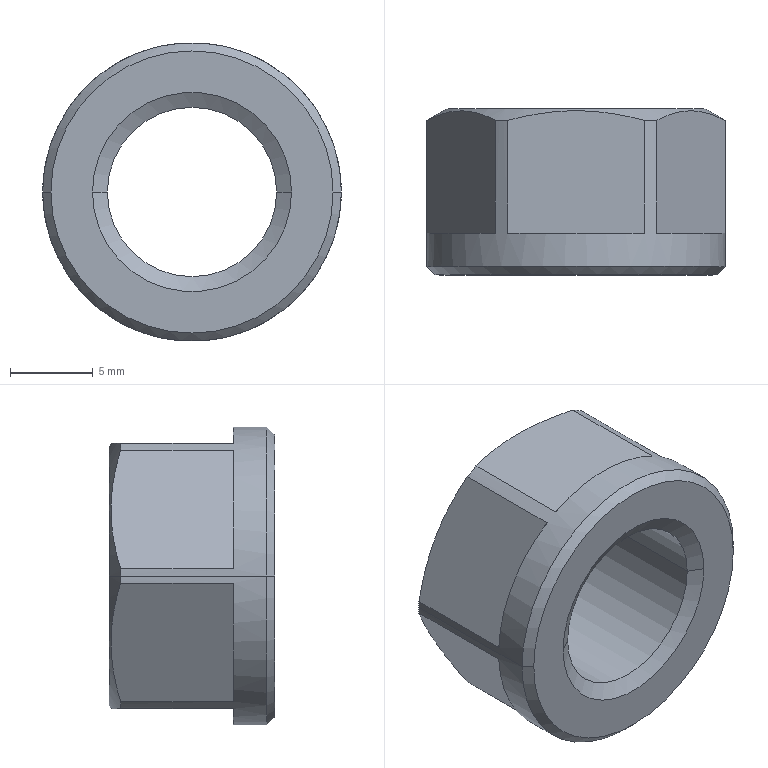Part | SolidWorks | features BaseBody 1 | 1 solid | 26 faces | box 18 x 10 x 18 mm | volume 1447 mm3 | plane 14 | cone 8 | cylinder 4 | commonest cylinder face diameters 10.2 x2 18 x2
STEP:
#1=CARTESIAN_POINT('',(59.,179.1,-24.25));
#2=VERTEX_POINT('',#1);
#3=CARTESIAN_POINT('',(42.,179.1,-24.25));
#4=VERTEX_POINT('',#3);
#5=CARTESIAN_POINT('',(50.5,179.1,-24.25));
#6=DIRECTION('',(0.,-1.,0.));
#7=DIRECTION('',(-1.,0.,0.));
#8=AXIS2_PLACEMENT_3D('',#5,#6,#7);
#9=CIRCLE('',#8,8.5);
#10=EDGE_CURVE('',#2,#4,#9,.T.);
#11=ORIENTED_EDGE('',*,*,#10,.F.);
#12=CARTESIAN_POINT('',(59.5,179.6,-24.25));
#13=VERTEX_POINT('',#12);
#14=CARTESIAN_POINT('',(59.5,179.6,-24.25));
#15=DIRECTION('',(0.7071,0.7071,0.));
#16=VECTOR('',#15,1000.);
#17=LINE('',#14,#16);
#18=EDGE_CURVE('',#2,#13,#17,.T.);
#19=ORIENTED_EDGE('',*,*,#18,.T.);
#20=CARTESIAN_POINT('',(41.5,179.6,-24.25));
#21=VERTEX_POINT('',#20);
#22=CARTESIAN_POINT('',(50.5,179.6,-24.25));
#23=DIRECTION('',(0.,1.,0.));
#24=DIRECTION('',(-1.,0.,0.));
#25=AXIS2_PLACEMENT_3D('',#22,#23,#24);
#26=CIRCLE('',#25,9.);
#27=EDGE_CURVE('',#21,#13,#26,.T.);
#28=ORIENTED_EDGE('',*,*,#27,.F.);
#29=CARTESIAN_POINT('',(41.5,179.6,-24.25));
#30=DIRECTION('',(-0.7071,0.7071,0.));
#31=VECTOR('',#30,1000.);
#32=LINE('',#29,#31);
#33=EDGE_CURVE('',#4,#21,#32,.T.);
#34=ORIENTED_EDGE('',*,*,#33,.F.);
#35=EDGE_LOOP('',(#11,#19,#28,#34));
#36=FACE_OUTER_BOUND('',#35,.T.);
#37=CARTESIAN_POINT('',(50.5,179.6,-24.25));
#38=DIRECTION('',(0.,1.,0.));
#39=DIRECTION('',(-1.,0.,0.));
#40=AXIS2_PLACEMENT_3D('',#37,#38,#39);
#41=CONICAL_SURFACE('',#40,9.,0.7854);
#42=ADVANCED_FACE('',(#36),#41,.T.);
#43=CARTESIAN_POINT('',(58.294,189.1,-24.25));
#44=VERTEX_POINT('',#43);
#45=CARTESIAN_POINT('',(42.706,189.1,-24.25));
#46=VERTEX_POINT('',#45);
#47=CARTESIAN_POINT('',(50.5,189.1,-24.25));
#48=DIRECTION('',(0.,1.,0.));
#49=DIRECTION('',(-1.,0.,0.));
#50=AXIS2_PLACEMENT_3D('',#47,#48,#49);
#51=CIRCLE('',#50,7.794);
#52=EDGE_CURVE('',#44,#46,#51,.T.);
#53=ORIENTED_EDGE('',*,*,#52,.F.);
#54=CARTESIAN_POINT('',(59.5,188.404,-24.25));
#55=VERTEX_POINT('',#54);
#56=CARTESIAN_POINT('',(58.294,189.1,-24.25));
#57=DIRECTION('',(0.866,-0.5,0.));
#58=VECTOR('',#57,1000.);
#59=LINE('',#56,#58);
#60=EDGE_CURVE('',#44,#55,#59,.T.);
#61=ORIENTED_EDGE('',*,*,#60,.T.);
#62=CARTESIAN_POINT('',(59.49,188.404,-24.679));
#63=VERTEX_POINT('',#62);
#64=CARTESIAN_POINT('',(50.5,188.404,-24.25));
#65=DIRECTION('',(0.,1.,0.));
#66=DIRECTION('',(1.,0.,0.));
#67=AXIS2_PLACEMENT_3D('',#64,#65,#66);
#68=CIRCLE('',#67,9.);
#69=EDGE_CURVE('',#55,#63,#68,.T.);
#70=ORIENTED_EDGE('',*,*,#69,.T.);
#71=CARTESIAN_POINT('',(55.367,188.404,-31.821));
#72=VERTEX_POINT('',#71);
#73=CARTESIAN_POINT('',(59.49,188.404,-24.679));
#74=CARTESIAN_POINT('',(59.152,188.582,-25.264));
#75=CARTESIAN_POINT('',(58.812,188.727,-25.852));
#76=CARTESIAN_POINT('',(58.128,188.927,-27.038));
#77=CARTESIAN_POINT('',(57.783,188.981,-27.636));
#78=CARTESIAN_POINT('',(57.261,188.982,-28.54));
#79=CARTESIAN_POINT('',(57.086,188.969,-28.843));
#80=CARTESIAN_POINT('',(56.737,188.917,-29.448));
#81=CARTESIAN_POINT('',(56.563,188.878,-29.748));
#82=CARTESIAN_POINT('',(56.046,188.728,-30.644));
#83=CARTESIAN_POINT('',(55.705,188.583,-31.235));
#84=CARTESIAN_POINT('',(55.367,188.404,-31.821));
#85=B_SPLINE_CURVE_WITH_KNOTS('',3,(#73,#74,#75,#76,#77,#78,#79,#80,#81,#82,#83,#84),.UNSPECIFIED.,.F.,.F.,(4,2,2,2,2,4),(0.000000296,0.002075,0.004149,0.005186,0.006223,0.008298),.UNSPECIFIED.);
#86=EDGE_CURVE('',#63,#72,#85,.T.);
#87=ORIENTED_EDGE('',*,*,#86,.T.);
#88=CARTESIAN_POINT('',(54.623,188.404,-32.25));
#89=VERTEX_POINT('',#88);
#90=CARTESIAN_POINT('',(50.5,188.404,-24.25));
#91=DIRECTION('',(0.,1.,0.));
#92=DIRECTION('',(1.,0.,0.));
#93=AXIS2_PLACEMENT_3D('',#90,#91,#92);
#94=CIRCLE('',#93,9.);
#95=EDGE_CURVE('',#72,#89,#94,.T.);
#96=ORIENTED_EDGE('',*,*,#95,.T.);
#97=CARTESIAN_POINT('',(46.377,188.404,-32.25));
#98=VERTEX_POINT('',#97);
#99=CARTESIAN_POINT('',(54.623,188.404,-32.25));
#100=CARTESIAN_POINT('',(53.948,188.582,-32.25));
#101=CARTESIAN_POINT('',(53.268,188.727,-32.25));
#102=CARTESIAN_POINT('',(51.899,188.927,-32.25));
#103=CARTESIAN_POINT('',(51.21,188.981,-32.25));
#104=CARTESIAN_POINT('',(50.166,188.982,-32.25));
#105=CARTESIAN_POINT('',(49.815,188.969,-32.25));
#106=CARTESIAN_POINT('',(49.117,188.917,-32.25));
#107=CARTESIAN_POINT('',(48.77,188.878,-32.25));
#108=CARTESIAN_POINT('',(47.736,188.728,-32.25));
#109=CARTESIAN_POINT('',(47.054,188.583,-32.25));
#110=CARTESIAN_POINT('',(46.377,188.404,-32.25));
#111=B_SPLINE_CURVE_WITH_KNOTS('',3,(#99,#100,#101,#102,#103,#104,#105,#106,#107,#108,#109,#110),.UNSPECIFIED.,.F.,.F.,(4,2,2,2,2,4),(0.000000256,0.002075,0.004149,0.005186,0.006223,0.008298),.UNSPECIFIED.);
#112=EDGE_CURVE('',#89,#98,#111,.T.);
#113=ORIENTED_EDGE('',*,*,#112,.T.);
#114=CARTESIAN_POINT('',(45.633,188.404,-31.821));
#115=VERTEX_POINT('',#114);
#116=CARTESIAN_POINT('',(50.5,188.404,-24.25));
#117=DIRECTION('',(0.,1.,0.));
#118=DIRECTION('',(1.,0.,0.));
#119=AXIS2_PLACEMENT_3D('',#116,#117,#118);
#120=CIRCLE('',#119,9.);
#121=EDGE_CURVE('',#98,#115,#120,.T.);
#122=ORIENTED_EDGE('',*,*,#121,.T.);
#123=CARTESIAN_POINT('',(41.51,188.404,-24.679));
#124=VERTEX_POINT('',#123);
#125=CARTESIAN_POINT('',(45.633,188.404,-31.821));
#126=CARTESIAN_POINT('',(45.296,188.582,-31.236));
#127=CARTESIAN_POINT('',(44.956,188.727,-30.648));
#128=CARTESIAN_POINT('',(44.271,188.927,-29.462));
#129=CARTESIAN_POINT('',(43.927,188.981,-28.864));
#130=CARTESIAN_POINT('',(43.405,188.982,-27.96));
#131=CARTESIAN_POINT('',(43.229,188.969,-27.657));
#132=CARTESIAN_POINT('',(42.88,188.917,-27.052));
#133=CARTESIAN_POINT('',(42.707,188.878,-26.752));
#134=CARTESIAN_POINT('',(42.19,188.728,-25.856));
#135=CARTESIAN_POINT('',(41.849,188.583,-25.265));
#136=CARTESIAN_POINT('',(41.51,188.404,-24.679));
#137=B_SPLINE_CURVE_WITH_KNOTS('',3,(#125,#126,#127,#128,#129,#130,#131,#132,#133,#134,#135,#136),.UNSPECIFIED.,.F.,.F.,(4,2,2,2,2,4),(0.000000296,0.002075,0.004149,0.005186,0.006223,0.008298),.UNSPECIFIED.);
#138=EDGE_CURVE('',#115,#124,#137,.T.);
#139=ORIENTED_EDGE('',*,*,#138,.T.);
#140=CARTESIAN_POINT('',(41.5,188.404,-24.25));
#141=VERTEX_POINT('',#140);
#142=CARTESIAN_POINT('',(50.5,188.404,-24.25));
#143=DIRECTION('',(0.,1.,0.));
#144=DIRECTION('',(1.,0.,0.));
#145=AXIS2_PLACEMENT_3D('',#142,#143,#144);
#146=CIRCLE('',#145,9.);
#147=EDGE_CURVE('',#124,#141,#146,.T.);
#148=ORIENTED_EDGE('',*,*,#147,.T.);
#149=CARTESIAN_POINT('',(42.706,189.1,-24.25));
#150=DIRECTION('',(-0.866,-0.5,0.));
#151=VECTOR('',#150,1000.);
#152=LINE('',#149,#151);
#153=EDGE_CURVE('',#46,#141,#152,.T.);
#154=ORIENTED_EDGE('',*,*,#153,.F.);
#155=EDGE_LOOP('',(#53,#61,#70,#87,#96,#113,#122,#139,#148,#154));
#156=FACE_OUTER_BOUND('',#155,.T.);
#157=CARTESIAN_POINT('',(50.5,189.1,-24.25));
#158=DIRECTION('',(0.,-1.,0.));
#159=DIRECTION('',(-1.,0.,0.));
#160=AXIS2_PLACEMENT_3D('',#157,#158,#159);
#161=CONICAL_SURFACE('',#160,7.794,1.047);
#162=ADVANCED_FACE('',(#156),#161,.T.);
#163=CARTESIAN_POINT('',(55.6,179.62,-24.25));
#164=VERTEX_POINT('',#163);
#165=CARTESIAN_POINT('',(45.4,179.62,-24.25));
#166=VERTEX_POINT('',#165);
#167=CARTESIAN_POINT('',(50.5,179.62,-24.25));
#168=DIRECTION('',(0.,1.,0.));
#169=DIRECTION('',(-1.,0.,0.));
#170=AXIS2_PLACEMENT_3D('',#167,#168,#169);
#171=CIRCLE('',#170,5.1);
#172=EDGE_CURVE('',#164,#166,#171,.T.);
#173=ORIENTED_EDGE('',*,*,#172,.T.);
#174=CARTESIAN_POINT('',(44.5,179.1,-24.25));
#175=VERTEX_POINT('',#174);
#176=CARTESIAN_POINT('',(45.4,179.62,-24.25));
#177=DIRECTION('',(-0.866,-0.5,0.));
#178=VECTOR('',#177,1000.);
#179=LINE('',#176,#178);
#180=EDGE_CURVE('',#166,#175,#179,.T.);
#181=ORIENTED_EDGE('',*,*,#180,.T.);
#182=CARTESIAN_POINT('',(56.5,179.1,-24.25));
#183=VERTEX_POINT('',#182);
#184=CARTESIAN_POINT('',(50.5,179.1,-24.25));
#185=DIRECTION('',(0.,1.,0.));
#186=DIRECTION('',(-1.,0.,0.));
#187=AXIS2_PLACEMENT_3D('',#184,#185,#186);
#188=CIRCLE('',#187,6.);
#189=EDGE_CURVE('',#183,#175,#188,.T.);
#190=ORIENTED_EDGE('',*,*,#189,.F.);
#191=CARTESIAN_POINT('',(55.6,179.62,-24.25));
#192=DIRECTION('',(0.866,-0.5,0.));
#193=VECTOR('',#192,1000.);
#194=LINE('',#191,#193);
#195=EDGE_CURVE('',#164,#183,#194,.T.);
#196=ORIENTED_EDGE('',*,*,#195,.F.);
#197=EDGE_LOOP('',(#173,#181,#190,#196));
#198=FACE_OUTER_BOUND('',#197,.T.);
#199=CARTESIAN_POINT('',(50.5,179.62,-24.25));
#200=DIRECTION('',(0.,-1.,0.));
#201=DIRECTION('',(1.,0.,0.));
#202=AXIS2_PLACEMENT_3D('',#199,#200,#201);
#203=CONICAL_SURFACE('',#202,5.1,1.047);
#204=ADVANCED_FACE('',(#198),#203,.F.);
#205=ORIENTED_EDGE('',*,*,#172,.F.);
#206=CARTESIAN_POINT('',(55.6,188.58,-24.25));
#207=VERTEX_POINT('',#206);
#208=CARTESIAN_POINT('',(55.6,189.1,-24.25));
#209=DIRECTION('',(0.,1.,0.));
#210=VECTOR('',#209,1000.);
#211=LINE('',#208,#210);
#212=EDGE_CURVE('',#164,#207,#211,.T.);
#213=ORIENTED_EDGE('',*,*,#212,.T.);
#214=CARTESIAN_POINT('',(45.4,188.58,-24.25));
#215=VERTEX_POINT('',#214);
#216=CARTESIAN_POINT('',(50.5,188.58,-24.25));
#217=DIRECTION('',(0.,1.,0.));
#218=DIRECTION('',(-1.,0.,0.));
#219=AXIS2_PLACEMENT_3D('',#216,#217,#218);
#220=CIRCLE('',#219,5.1);
#221=EDGE_CURVE('',#207,#215,#220,.T.);
#222=ORIENTED_EDGE('',*,*,#221,.T.);
#223=CARTESIAN_POINT('',(45.4,189.1,-24.25));
#224=DIRECTION('',(0.,1.,0.));
#225=VECTOR('',#224,1000.);
#226=LINE('',#223,#225);
#227=EDGE_CURVE('',#166,#215,#226,.T.);
#228=ORIENTED_EDGE('',*,*,#227,.F.);
#229=EDGE_LOOP('',(#205,#213,#222,#228));
#230=FACE_OUTER_BOUND('',#229,.T.);
#231=CARTESIAN_POINT('',(50.5,189.1,-24.25));
#232=DIRECTION('',(0.,1.,0.));
#233=DIRECTION('',(-1.,0.,0.));
#234=AXIS2_PLACEMENT_3D('',#231,#232,#233);
#235=CYLINDRICAL_SURFACE('',#234,5.1);
#236=ADVANCED_FACE('',(#230),#235,.F.);
#237=ORIENTED_EDGE('',*,*,#221,.F.);
#238=CARTESIAN_POINT('',(56.5,189.1,-24.25));
#239=VERTEX_POINT('',#238);
#240=CARTESIAN_POINT('',(56.5,189.1,-24.25));
#241=DIRECTION('',(0.866,0.5,0.));
#242=VECTOR('',#241,1000.);
#243=LINE('',#240,#242);
#244=EDGE_CURVE('',#207,#239,#243,.T.);
#245=ORIENTED_EDGE('',*,*,#244,.T.);
#246=CARTESIAN_POINT('',(44.5,189.1,-24.25));
#247=VERTEX_POINT('',#246);
#248=CARTESIAN_POINT('',(50.5,189.1,-24.25));
#249=DIRECTION('',(0.,1.,0.));
#250=DIRECTION('',(-1.,0.,0.));
#251=AXIS2_PLACEMENT_3D('',#248,#249,#250);
#252=CIRCLE('',#251,6.);
#253=EDGE_CURVE('',#239,#247,#252,.T.);
#254=ORIENTED_EDGE('',*,*,#253,.T.);
#255=CARTESIAN_POINT('',(44.5,189.1,-24.25));
#256=DIRECTION('',(-0.866,0.5,0.));
#257=VECTOR('',#256,1000.);
#258=LINE('',#255,#257);
#259=EDGE_CURVE('',#215,#247,#258,.T.);
#260=ORIENTED_EDGE('',*,*,#259,.F.);
#261=EDGE_LOOP('',(#237,#245,#254,#260));
#262=FACE_OUTER_BOUND('',#261,.T.);
#263=CARTESIAN_POINT('',(50.5,189.1,-24.25));
#264=DIRECTION('',(0.,1.,0.));
#265=DIRECTION('',(-1.,0.,0.));
#266=AXIS2_PLACEMENT_3D('',#263,#264,#265);
#267=CONICAL_SURFACE('',#266,6.,1.047);
#268=ADVANCED_FACE('',(#262),#267,.F.);
#269=CARTESIAN_POINT('',(41.51,188.404,-23.821));
#270=VERTEX_POINT('',#269);
#271=CARTESIAN_POINT('',(50.5,188.404,-24.25));
#272=DIRECTION('',(0.,1.,0.));
#273=DIRECTION('',(1.,0.,0.));
#274=AXIS2_PLACEMENT_3D('',#271,#272,#273);
#275=CIRCLE('',#274,9.);
#276=EDGE_CURVE('',#141,#270,#275,.T.);
#277=ORIENTED_EDGE('',*,*,#276,.F.);
#278=CARTESIAN_POINT('',(41.5,181.6,-24.25));
#279=DIRECTION('',(0.,-1.,0.));
#280=VECTOR('',#279,1000.);
#281=LINE('',#278,#280);
#282=EDGE_CURVE('',#141,#21,#281,.T.);
#283=ORIENTED_EDGE('',*,*,#282,.T.);
#284=ORIENTED_EDGE('',*,*,#27,.T.);
#285=CARTESIAN_POINT('',(59.5,181.6,-24.25));
#286=DIRECTION('',(0.,-1.,0.));
#287=VECTOR('',#286,1000.);
#288=LINE('',#285,#287);
#289=EDGE_CURVE('',#55,#13,#288,.T.);
#290=ORIENTED_EDGE('',*,*,#289,.F.);
#291=CARTESIAN_POINT('',(59.49,188.404,-23.821));
#292=VERTEX_POINT('',#291);
#293=CARTESIAN_POINT('',(50.5,188.404,-24.25));
#294=DIRECTION('',(0.,1.,0.));
#295=DIRECTION('',(1.,0.,0.));
#296=AXIS2_PLACEMENT_3D('',#293,#294,#295);
#297=CIRCLE('',#296,9.);
#298=EDGE_CURVE('',#292,#55,#297,.T.);
#299=ORIENTED_EDGE('',*,*,#298,.F.);
#300=CARTESIAN_POINT('',(59.49,181.6,-23.821));
#301=VERTEX_POINT('',#300);
#302=CARTESIAN_POINT('',(59.49,223.183,-23.821));
#303=DIRECTION('',(0.,-1.,0.));
#304=VECTOR('',#303,1000.);
#305=LINE('',#302,#304);
#306=EDGE_CURVE('',#292,#301,#305,.T.);
#307=ORIENTED_EDGE('',*,*,#306,.T.);
#308=CARTESIAN_POINT('',(55.367,181.6,-16.679));
#309=VERTEX_POINT('',#308);
#310=CARTESIAN_POINT('',(50.5,181.6,-24.25));
#311=DIRECTION('',(0.,1.,0.));
#312=DIRECTION('',(-1.,0.,0.));
#313=AXIS2_PLACEMENT_3D('',#310,#311,#312);
#314=CIRCLE('',#313,9.);
#315=EDGE_CURVE('',#309,#301,#314,.T.);
#316=ORIENTED_EDGE('',*,*,#315,.F.);
#317=CARTESIAN_POINT('',(55.367,188.404,-16.679));
#318=VERTEX_POINT('',#317);
#319=CARTESIAN_POINT('',(55.367,223.183,-16.679));
#320=DIRECTION('',(0.,-1.,0.));
#321=VECTOR('',#320,1000.);
#322=LINE('',#319,#321);
#323=EDGE_CURVE('',#318,#309,#322,.T.);
#324=ORIENTED_EDGE('',*,*,#323,.F.);
#325=CARTESIAN_POINT('',(54.623,188.404,-16.25));
#326=VERTEX_POINT('',#325);
#327=CARTESIAN_POINT('',(50.5,188.404,-24.25));
#328=DIRECTION('',(0.,1.,0.));
#329=DIRECTION('',(1.,0.,0.));
#330=AXIS2_PLACEMENT_3D('',#327,#328,#329);
#331=CIRCLE('',#330,9.);
#332=EDGE_CURVE('',#326,#318,#331,.T.);
#333=ORIENTED_EDGE('',*,*,#332,.F.);
#334=CARTESIAN_POINT('',(54.623,181.6,-16.25));
#335=VERTEX_POINT('',#334);
#336=CARTESIAN_POINT('',(54.623,223.183,-16.25));
#337=DIRECTION('',(0.,-1.,0.));
#338=VECTOR('',#337,1000.);
#339=LINE('',#336,#338);
#340=EDGE_CURVE('',#326,#335,#339,.T.);
#341=ORIENTED_EDGE('',*,*,#340,.T.);
#342=CARTESIAN_POINT('',(46.377,181.6,-16.25));
#343=VERTEX_POINT('',#342);
#344=CARTESIAN_POINT('',(50.5,181.6,-24.25));
#345=DIRECTION('',(0.,1.,0.));
#346=DIRECTION('',(-1.,0.,0.));
#347=AXIS2_PLACEMENT_3D('',#344,#345,#346);
#348=CIRCLE('',#347,9.);
#349=EDGE_CURVE('',#343,#335,#348,.T.);
#350=ORIENTED_EDGE('',*,*,#349,.F.);
#351=CARTESIAN_POINT('',(46.377,188.404,-16.25));
#352=VERTEX_POINT('',#351);
#353=CARTESIAN_POINT('',(46.377,223.183,-16.25));
#354=DIRECTION('',(0.,-1.,0.));
#355=VECTOR('',#354,1000.);
#356=LINE('',#353,#355);
#357=EDGE_CURVE('',#352,#343,#356,.T.);
#358=ORIENTED_EDGE('',*,*,#357,.F.);
#359=CARTESIAN_POINT('',(45.633,188.404,-16.679));
#360=VERTEX_POINT('',#359);
#361=CARTESIAN_POINT('',(50.5,188.404,-24.25));
#362=DIRECTION('',(0.,1.,0.));
#363=DIRECTION('',(1.,0.,0.));
#364=AXIS2_PLACEMENT_3D('',#361,#362,#363);
#365=CIRCLE('',#364,9.);
#366=EDGE_CURVE('',#360,#352,#365,.T.);
#367=ORIENTED_EDGE('',*,*,#366,.F.);
#368=CARTESIAN_POINT('',(45.633,181.6,-16.679));
#369=VERTEX_POINT('',#368);
#370=CARTESIAN_POINT('',(45.633,223.183,-16.679));
#371=DIRECTION('',(0.,-1.,0.));
#372=VECTOR('',#371,1000.);
#373=LINE('',#370,#372);
#374=EDGE_CURVE('',#360,#369,#373,.T.);
#375=ORIENTED_EDGE('',*,*,#374,.T.);
#376=CARTESIAN_POINT('',(41.51,181.6,-23.821));
#377=VERTEX_POINT('',#376);
#378=CARTESIAN_POINT('',(50.5,181.6,-24.25));
#379=DIRECTION('',(0.,1.,0.));
#380=DIRECTION('',(-1.,0.,0.));
#381=AXIS2_PLACEMENT_3D('',#378,#379,#380);
#382=CIRCLE('',#381,9.);
#383=EDGE_CURVE('',#377,#369,#382,.T.);
#384=ORIENTED_EDGE('',*,*,#383,.F.);
#385=CARTESIAN_POINT('',(41.51,223.183,-23.821));
#386=DIRECTION('',(0.,-1.,0.));
#387=VECTOR('',#386,1000.);
#388=LINE('',#385,#387);
#389=EDGE_CURVE('',#270,#377,#388,.T.);
#390=ORIENTED_EDGE('',*,*,#389,.F.);
#391=EDGE_LOOP('',(#277,#283,#284,#290,#299,#307,#316,#324,#333,#341,#350,#358,#367,#375,#384,#390));
#392=FACE_OUTER_BOUND('',#391,.T.);
#393=CARTESIAN_POINT('',(50.5,181.6,-24.25));
#394=DIRECTION('',(0.,-1.,0.));
#395=DIRECTION('',(1.,0.,0.));
#396=AXIS2_PLACEMENT_3D('',#393,#394,#395);
#397=CYLINDRICAL_SURFACE('',#396,9.);
#398=ADVANCED_FACE('',(#392),#397,.T.);
#399=ORIENTED_EDGE('',*,*,#282,.F.);
#400=ORIENTED_EDGE('',*,*,#147,.F.);
#401=CARTESIAN_POINT('',(41.51,181.6,-24.679));
#402=VERTEX_POINT('',#401);
#403=CARTESIAN_POINT('',(41.51,223.183,-24.679));
#404=DIRECTION('',(0.,-1.,0.));
#405=VECTOR('',#404,1000.);
#406=LINE('',#403,#405);
#407=EDGE_CURVE('',#124,#402,#406,.T.);
#408=ORIENTED_EDGE('',*,*,#407,.T.);
#409=CARTESIAN_POINT('',(45.633,181.6,-31.821));
#410=VERTEX_POINT('',#409);
#411=CARTESIAN_POINT('',(50.5,181.6,-24.25));
#412=DIRECTION('',(0.,1.,0.));
#413=DIRECTION('',(-1.,0.,0.));
#414=AXIS2_PLACEMENT_3D('',#411,#412,#413);
#415=CIRCLE('',#414,9.);
#416=EDGE_CURVE('',#410,#402,#415,.T.);
#417=ORIENTED_EDGE('',*,*,#416,.F.);
#418=CARTESIAN_POINT('',(45.633,223.183,-31.821));
#419=DIRECTION('',(0.,-1.,0.));
#420=VECTOR('',#419,1000.);
#421=LINE('',#418,#420);
#422=EDGE_CURVE('',#115,#410,#421,.T.);
#423=ORIENTED_EDGE('',*,*,#422,.F.);
#424=ORIENTED_EDGE('',*,*,#121,.F.);
#425=CARTESIAN_POINT('',(46.377,181.6,-32.25));
#426=VERTEX_POINT('',#425);
#427=CARTESIAN_POINT('',(46.377,223.183,-32.25));
#428=DIRECTION('',(0.,-1.,0.));
#429=VECTOR('',#428,1000.);
#430=LINE('',#427,#429);
#431=EDGE_CURVE('',#98,#426,#430,.T.);
#432=ORIENTED_EDGE('',*,*,#431,.T.);
#433=CARTESIAN_POINT('',(54.623,181.6,-32.25));
#434=VERTEX_POINT('',#433);
#435=CARTESIAN_POINT('',(50.5,181.6,-24.25));
#436=DIRECTION('',(0.,1.,0.));
#437=DIRECTION('',(-1.,0.,0.));
#438=AXIS2_PLACEMENT_3D('',#435,#436,#437);
#439=CIRCLE('',#438,9.);
#440=EDGE_CURVE('',#434,#426,#439,.T.);
#441=ORIENTED_EDGE('',*,*,#440,.F.);
#442=CARTESIAN_POINT('',(54.623,223.183,-32.25));
#443=DIRECTION('',(0.,-1.,0.));
#444=VECTOR('',#443,1000.);
#445=LINE('',#442,#444);
#446=EDGE_CURVE('',#89,#434,#445,.T.);
#447=ORIENTED_EDGE('',*,*,#446,.F.);
#448=ORIENTED_EDGE('',*,*,#95,.F.);
#449=CARTESIAN_POINT('',(55.367,181.6,-31.821));
#450=VERTEX_POINT('',#449);
#451=CARTESIAN_POINT('',(55.367,223.183,-31.821));
#452=DIRECTION('',(0.,-1.,0.));
#453=VECTOR('',#452,1000.);
#454=LINE('',#451,#453);
#455=EDGE_CURVE('',#72,#450,#454,.T.);
#456=ORIENTED_EDGE('',*,*,#455,.T.);
#457=CARTESIAN_POINT('',(59.49,181.6,-24.679));
#458=VERTEX_POINT('',#457);
#459=CARTESIAN_POINT('',(50.5,181.6,-24.25));
#460=DIRECTION('',(0.,1.,0.));
#461=DIRECTION('',(-1.,0.,0.));
#462=AXIS2_PLACEMENT_3D('',#459,#460,#461);
#463=CIRCLE('',#462,9.);
#464=EDGE_CURVE('',#458,#450,#463,.T.);
#465=ORIENTED_EDGE('',*,*,#464,.F.);
#466=CARTESIAN_POINT('',(59.49,223.183,-24.679));
#467=DIRECTION('',(0.,-1.,0.));
#468=VECTOR('',#467,1000.);
#469=LINE('',#466,#468);
#470=EDGE_CURVE('',#63,#458,#469,.T.);
#471=ORIENTED_EDGE('',*,*,#470,.F.);
#472=ORIENTED_EDGE('',*,*,#69,.F.);
#473=ORIENTED_EDGE('',*,*,#289,.T.);
#474=CARTESIAN_POINT('',(50.5,179.6,-24.25));
#475=DIRECTION('',(0.,1.,0.));
#476=DIRECTION('',(-1.,0.,0.));
#477=AXIS2_PLACEMENT_3D('',#474,#475,#476);
#478=CIRCLE('',#477,9.);
#479=EDGE_CURVE('',#13,#21,#478,.T.);
#480=ORIENTED_EDGE('',*,*,#479,.T.);
#481=EDGE_LOOP('',(#399,#400,#408,#417,#423,#424,#432,#441,#447,#448,#456,#465,#471,#472,#473,#480));
#482=FACE_OUTER_BOUND('',#481,.T.);
#483=CARTESIAN_POINT('',(50.5,181.6,-24.25));
#484=DIRECTION('',(0.,-1.,0.));
#485=DIRECTION('',(1.,0.,0.));
#486=AXIS2_PLACEMENT_3D('',#483,#484,#485);
#487=CYLINDRICAL_SURFACE('',#486,9.);
#488=ADVANCED_FACE('',(#482),#487,.T.);
#489=CARTESIAN_POINT('',(46.377,188.404,-16.25));
#490=CARTESIAN_POINT('',(47.052,188.582,-16.25));
#491=CARTESIAN_POINT('',(47.732,188.727,-16.25));
#492=CARTESIAN_POINT('',(49.101,188.927,-16.25));
#493=CARTESIAN_POINT('',(49.79,188.981,-16.25));
#494=CARTESIAN_POINT('',(50.834,188.982,-16.25));
#495=CARTESIAN_POINT('',(51.185,188.969,-16.25));
#496=CARTESIAN_POINT('',(51.883,188.917,-16.25));
#497=CARTESIAN_POINT('',(52.23,188.878,-16.25));
#498=CARTESIAN_POINT('',(53.264,188.728,-16.25));
#499=CARTESIAN_POINT('',(53.946,188.583,-16.25));
#500=CARTESIAN_POINT('',(54.623,188.404,-16.25));
#501=B_SPLINE_CURVE_WITH_KNOTS('',3,(#489,#490,#491,#492,#493,#494,#495,#496,#497,#498,#499,#500),.UNSPECIFIED.,.F.,.F.,(4,2,2,2,2,4),(0.000000256,0.002075,0.004149,0.005186,0.006223,0.008298),.UNSPECIFIED.);
#502=EDGE_CURVE('',#352,#326,#501,.T.);
#503=ORIENTED_EDGE('',*,*,#502,.F.);
#504=ORIENTED_EDGE('',*,*,#357,.T.);
#505=CARTESIAN_POINT('',(46.377,181.6,-16.25));
#506=DIRECTION('',(1.,0.,0.));
#507=VECTOR('',#506,1000.);
#508=LINE('',#505,#507);
#509=EDGE_CURVE('',#343,#335,#508,.T.);
#510=ORIENTED_EDGE('',*,*,#509,.T.);
#511=ORIENTED_EDGE('',*,*,#340,.F.);
#512=EDGE_LOOP('',(#503,#504,#510,#511));
#513=FACE_OUTER_BOUND('',#512,.T.);
#514=CARTESIAN_POINT('',(46.377,223.183,-16.25));
#515=DIRECTION('',(0.,0.,-1.));
#516=DIRECTION('',(-1.,0.,0.));
#517=AXIS2_PLACEMENT_3D('',#514,#515,#516);
#518=PLANE('',#517);
#519=ADVANCED_FACE('',(#513),#518,.F.);
#520=CARTESIAN_POINT('',(55.367,188.404,-16.679));
#521=CARTESIAN_POINT('',(55.704,188.582,-17.264));
#522=CARTESIAN_POINT('',(56.044,188.727,-17.852));
#523=CARTESIAN_POINT('',(56.729,188.927,-19.038));
#524=CARTESIAN_POINT('',(57.073,188.981,-19.636));
#525=CARTESIAN_POINT('',(57.595,188.982,-20.54));
#526=CARTESIAN_POINT('',(57.771,188.969,-20.843));
#527=CARTESIAN_POINT('',(58.12,188.917,-21.448));
#528=CARTESIAN_POINT('',(58.293,188.878,-21.748));
#529=CARTESIAN_POINT('',(58.81,188.728,-22.644));
#530=CARTESIAN_POINT('',(59.151,188.583,-23.235));
#531=CARTESIAN_POINT('',(59.49,188.404,-23.821));
#532=B_SPLINE_CURVE_WITH_KNOTS('',3,(#520,#521,#522,#523,#524,#525,#526,#527,#528,#529,#530,#531),.UNSPECIFIED.,.F.,.F.,(4,2,2,2,2,4),(0.000000296,0.002075,0.004149,0.005186,0.006223,0.008298),.UNSPECIFIED.);
#533=EDGE_CURVE('',#318,#292,#532,.T.);
#534=ORIENTED_EDGE('',*,*,#533,.F.);
#535=ORIENTED_EDGE('',*,*,#323,.T.);
#536=CARTESIAN_POINT('',(55.367,181.6,-16.679));
#537=DIRECTION('',(0.5,0.,-0.866));
#538=VECTOR('',#537,1000.);
#539=LINE('',#536,#538);
#540=EDGE_CURVE('',#309,#301,#539,.T.);
#541=ORIENTED_EDGE('',*,*,#540,.T.);
#542=ORIENTED_EDGE('',*,*,#306,.F.);
#543=EDGE_LOOP('',(#534,#535,#541,#542));
#544=FACE_OUTER_BOUND('',#543,.T.);
#545=CARTESIAN_POINT('',(55.367,223.183,-16.679));
#546=DIRECTION('',(-0.866,0.,-0.5));
#547=DIRECTION('',(-0.5,0.,0.866));
#548=AXIS2_PLACEMENT_3D('',#545,#546,#547);
#549=PLANE('',#548);
#550=ADVANCED_FACE('',(#544),#549,.F.);
#551=ORIENTED_EDGE('',*,*,#86,.F.);
#552=ORIENTED_EDGE('',*,*,#470,.T.);
#553=CARTESIAN_POINT('',(59.49,181.6,-24.679));
#554=DIRECTION('',(-0.5,0.,-0.866));
#555=VECTOR('',#554,1000.);
#556=LINE('',#553,#555);
#557=EDGE_CURVE('',#458,#450,#556,.T.);
#558=ORIENTED_EDGE('',*,*,#557,.T.);
#559=ORIENTED_EDGE('',*,*,#455,.F.);
#560=EDGE_LOOP('',(#551,#552,#558,#559));
#561=FACE_OUTER_BOUND('',#560,.T.);
#562=CARTESIAN_POINT('',(59.49,223.183,-24.679));
#563=DIRECTION('',(-0.866,0.,0.5));
#564=DIRECTION('',(0.5,0.,0.866));
#565=AXIS2_PLACEMENT_3D('',#562,#563,#564);
#566=PLANE('',#565);
#567=ADVANCED_FACE('',(#561),#566,.F.);
#568=ORIENTED_EDGE('',*,*,#112,.F.);
#569=ORIENTED_EDGE('',*,*,#446,.T.);
#570=CARTESIAN_POINT('',(54.623,181.6,-32.25));
#571=DIRECTION('',(-1.,0.,0.));
#572=VECTOR('',#571,1000.);
#573=LINE('',#570,#572);
#574=EDGE_CURVE('',#434,#426,#573,.T.);
#575=ORIENTED_EDGE('',*,*,#574,.T.);
#576=ORIENTED_EDGE('',*,*,#431,.F.);
#577=EDGE_LOOP('',(#568,#569,#575,#576));
#578=FACE_OUTER_BOUND('',#577,.T.);
#579=CARTESIAN_POINT('',(54.623,223.183,-32.25));
#580=DIRECTION('',(0.,0.,1.));
#581=DIRECTION('',(0.,1.,0.));
#582=AXIS2_PLACEMENT_3D('',#579,#580,#581);
#583=PLANE('',#582);
#584=ADVANCED_FACE('',(#578),#583,.F.);
#585=ORIENTED_EDGE('',*,*,#138,.F.);
#586=ORIENTED_EDGE('',*,*,#422,.T.);
#587=CARTESIAN_POINT('',(45.633,181.6,-31.821));
#588=DIRECTION('',(-0.5,0.,0.866));
#589=VECTOR('',#588,1000.);
#590=LINE('',#587,#589);
#591=EDGE_CURVE('',#410,#402,#590,.T.);
#592=ORIENTED_EDGE('',*,*,#591,.T.);
#593=ORIENTED_EDGE('',*,*,#407,.F.);
#594=EDGE_LOOP('',(#585,#586,#592,#593));
#595=FACE_OUTER_BOUND('',#594,.T.);
#596=CARTESIAN_POINT('',(45.633,223.183,-31.821));
#597=DIRECTION('',(0.866,0.,0.5));
#598=DIRECTION('',(0.5,0.,-0.866));
#599=AXIS2_PLACEMENT_3D('',#596,#597,#598);
#600=PLANE('',#599);
#601=ADVANCED_FACE('',(#595),#600,.F.);
#602=CARTESIAN_POINT('',(41.51,188.404,-23.821));
#603=CARTESIAN_POINT('',(41.848,188.582,-23.236));
#604=CARTESIAN_POINT('',(42.188,188.727,-22.648));
#605=CARTESIAN_POINT('',(42.872,188.927,-21.462));
#606=CARTESIAN_POINT('',(43.217,188.981,-20.864));
#607=CARTESIAN_POINT('',(43.739,188.982,-19.96));
#608=CARTESIAN_POINT('',(43.914,188.969,-19.657));
#609=CARTESIAN_POINT('',(44.263,188.917,-19.052));
#610=CARTESIAN_POINT('',(44.437,188.878,-18.752));
#611=CARTESIAN_POINT('',(44.954,188.728,-17.856));
#612=CARTESIAN_POINT('',(45.295,188.583,-17.265));
#613=CARTESIAN_POINT('',(45.633,188.404,-16.679));
#614=B_SPLINE_CURVE_WITH_KNOTS('',3,(#602,#603,#604,#605,#606,#607,#608,#609,#610,#611,#612,#613),.UNSPECIFIED.,.F.,.F.,(4,2,2,2,2,4),(0.000000296,0.002075,0.004149,0.005186,0.006223,0.008298),.UNSPECIFIED.);
#615=EDGE_CURVE('',#270,#360,#614,.T.);
#616=ORIENTED_EDGE('',*,*,#615,.F.);
#617=ORIENTED_EDGE('',*,*,#389,.T.);
#618=CARTESIAN_POINT('',(41.51,181.6,-23.821));
#619=DIRECTION('',(0.5,0.,0.866));
#620=VECTOR('',#619,1000.);
#621=LINE('',#618,#620);
#622=EDGE_CURVE('',#377,#369,#621,.T.);
#623=ORIENTED_EDGE('',*,*,#622,.T.);
#624=ORIENTED_EDGE('',*,*,#374,.F.);
#625=EDGE_LOOP('',(#616,#617,#623,#624));
#626=FACE_OUTER_BOUND('',#625,.T.);
#627=CARTESIAN_POINT('',(41.51,223.183,-23.821));
#628=DIRECTION('',(0.866,0.,-0.5));
#629=DIRECTION('',(-0.5,0.,-0.866));
#630=AXIS2_PLACEMENT_3D('',#627,#628,#629);
#631=PLANE('',#630);
#632=ADVANCED_FACE('',(#626),#631,.F.);
#633=CARTESIAN_POINT('',(50.5,189.1,-24.25));
#634=DIRECTION('',(0.,1.,0.));
#635=DIRECTION('',(-1.,0.,0.));
#636=AXIS2_PLACEMENT_3D('',#633,#634,#635);
#637=CIRCLE('',#636,6.);
#638=EDGE_CURVE('',#247,#239,#637,.T.);
#639=ORIENTED_EDGE('',*,*,#638,.F.);
#640=ORIENTED_EDGE('',*,*,#253,.F.);
#641=EDGE_LOOP('',(#639,#640));
#642=FACE_BOUND('',#641,.T.);
#643=CARTESIAN_POINT('',(50.5,189.1,-24.25));
#644=DIRECTION('',(0.,1.,0.));
#645=DIRECTION('',(-1.,0.,0.));
#646=AXIS2_PLACEMENT_3D('',#643,#644,#645);
#647=CIRCLE('',#646,7.794);
#648=EDGE_CURVE('',#46,#44,#647,.T.);
#649=ORIENTED_EDGE('',*,*,#648,.T.);
#650=ORIENTED_EDGE('',*,*,#52,.T.);
#651=EDGE_LOOP('',(#649,#650));
#652=FACE_OUTER_BOUND('',#651,.T.);
#653=CARTESIAN_POINT('',(50.5,189.1,-24.25));
#654=DIRECTION('',(0.,1.,0.));
#655=DIRECTION('',(-1.,0.,0.));
#656=AXIS2_PLACEMENT_3D('',#653,#654,#655);
#657=PLANE('',#656);
#658=ADVANCED_FACE('',(#642,#652),#657,.T.);
#659=ORIENTED_EDGE('',*,*,#622,.F.);
#660=ORIENTED_EDGE('',*,*,#383,.T.);
#661=EDGE_LOOP('',(#659,#660));
#662=FACE_OUTER_BOUND('',#661,.T.);
#663=CARTESIAN_POINT('',(50.5,181.6,-24.25));
#664=DIRECTION('',(0.,1.,0.));
#665=DIRECTION('',(-1.,0.,0.));
#666=AXIS2_PLACEMENT_3D('',#663,#664,#665);
#667=PLANE('',#666);
#668=ADVANCED_FACE('',(#662),#667,.T.);
#669=ORIENTED_EDGE('',*,*,#591,.F.);
#670=ORIENTED_EDGE('',*,*,#416,.T.);
#671=EDGE_LOOP('',(#669,#670));
#672=FACE_OUTER_BOUND('',#671,.T.);
#673=CARTESIAN_POINT('',(50.5,181.6,-24.25));
#674=DIRECTION('',(0.,1.,0.));
#675=DIRECTION('',(-1.,0.,0.));
#676=AXIS2_PLACEMENT_3D('',#673,#674,#675);
#677=PLANE('',#676);
#678=ADVANCED_FACE('',(#672),#677,.T.);
#679=ORIENTED_EDGE('',*,*,#574,.F.);
#680=ORIENTED_EDGE('',*,*,#440,.T.);
#681=EDGE_LOOP('',(#679,#680));
#682=FACE_OUTER_BOUND('',#681,.T.);
#683=CARTESIAN_POINT('',(50.5,181.6,-24.25));
#684=DIRECTION('',(0.,1.,0.));
#685=DIRECTION('',(-1.,0.,0.));
#686=AXIS2_PLACEMENT_3D('',#683,#684,#685);
#687=PLANE('',#686);
#688=ADVANCED_FACE('',(#682),#687,.T.);
#689=ORIENTED_EDGE('',*,*,#557,.F.);
#690=ORIENTED_EDGE('',*,*,#464,.T.);
#691=EDGE_LOOP('',(#689,#690));
#692=FACE_OUTER_BOUND('',#691,.T.);
#693=CARTESIAN_POINT('',(50.5,181.6,-24.25));
#694=DIRECTION('',(0.,1.,0.));
#695=DIRECTION('',(-1.,0.,0.));
#696=AXIS2_PLACEMENT_3D('',#693,#694,#695);
#697=PLANE('',#696);
#698=ADVANCED_FACE('',(#692),#697,.T.);
#699=ORIENTED_EDGE('',*,*,#540,.F.);
#700=ORIENTED_EDGE('',*,*,#315,.T.);
#701=EDGE_LOOP('',(#699,#700));
#702=FACE_OUTER_BOUND('',#701,.T.);
#703=CARTESIAN_POINT('',(50.5,181.6,-24.25));
#704=DIRECTION('',(0.,1.,0.));
#705=DIRECTION('',(-1.,0.,0.));
#706=AXIS2_PLACEMENT_3D('',#703,#704,#705);
#707=PLANE('',#706);
#708=ADVANCED_FACE('',(#702),#707,.T.);
#709=ORIENTED_EDGE('',*,*,#509,.F.);
#710=ORIENTED_EDGE('',*,*,#349,.T.);
#711=EDGE_LOOP('',(#709,#710));
#712=FACE_OUTER_BOUND('',#711,.T.);
#713=CARTESIAN_POINT('',(50.5,181.6,-24.25));
#714=DIRECTION('',(0.,1.,0.));
#715=DIRECTION('',(-1.,0.,0.));
#716=AXIS2_PLACEMENT_3D('',#713,#714,#715);
#717=PLANE('',#716);
#718=ADVANCED_FACE('',(#712),#717,.T.);
#719=CARTESIAN_POINT('',(50.5,179.1,-24.25));
#720=DIRECTION('',(0.,-1.,0.));
#721=DIRECTION('',(-1.,0.,0.));
#722=AXIS2_PLACEMENT_3D('',#719,#720,#721);
#723=CIRCLE('',#722,8.5);
#724=EDGE_CURVE('',#4,#2,#723,.T.);
#725=ORIENTED_EDGE('',*,*,#724,.T.);
#726=ORIENTED_EDGE('',*,*,#10,.T.);
#727=EDGE_LOOP('',(#725,#726));
#728=FACE_OUTER_BOUND('',#727,.T.);
#729=ORIENTED_EDGE('',*,*,#189,.T.);
#730=CARTESIAN_POINT('',(50.5,179.1,-24.25));
#731=DIRECTION('',(0.,1.,0.));
#732=DIRECTION('',(-1.,0.,0.));
#733=AXIS2_PLACEMENT_3D('',#730,#731,#732);
#734=CIRCLE('',#733,6.);
#735=EDGE_CURVE('',#175,#183,#734,.T.);
#736=ORIENTED_EDGE('',*,*,#735,.T.);
#737=EDGE_LOOP('',(#729,#736));
#738=FACE_BOUND('',#737,.T.);
#739=CARTESIAN_POINT('',(50.5,179.1,-24.25));
#740=DIRECTION('',(0.,1.,0.));
#741=DIRECTION('',(-1.,0.,0.));
#742=AXIS2_PLACEMENT_3D('',#739,#740,#741);
#743=PLANE('',#742);
#744=ADVANCED_FACE('',(#728,#738),#743,.F.);
#745=ORIENTED_EDGE('',*,*,#244,.F.);
#746=CARTESIAN_POINT('',(50.5,188.58,-24.25));
#747=DIRECTION('',(0.,1.,0.));
#748=DIRECTION('',(-1.,0.,0.));
#749=AXIS2_PLACEMENT_3D('',#746,#747,#748);
#750=CIRCLE('',#749,5.1);
#751=EDGE_CURVE('',#215,#207,#750,.T.);
#752=ORIENTED_EDGE('',*,*,#751,.F.);
#753=ORIENTED_EDGE('',*,*,#259,.T.);
#754=ORIENTED_EDGE('',*,*,#638,.T.);
#755=EDGE_LOOP('',(#745,#752,#753,#754));
#756=FACE_OUTER_BOUND('',#755,.T.);
#757=CARTESIAN_POINT('',(50.5,189.1,-24.25));
#758=DIRECTION('',(0.,1.,0.));
#759=DIRECTION('',(-1.,0.,0.));
#760=AXIS2_PLACEMENT_3D('',#757,#758,#759);
#761=CONICAL_SURFACE('',#760,6.,1.047);
#762=ADVANCED_FACE('',(#756),#761,.F.);
#763=ORIENTED_EDGE('',*,*,#212,.F.);
#764=CARTESIAN_POINT('',(50.5,179.62,-24.25));
#765=DIRECTION('',(0.,1.,0.));
#766=DIRECTION('',(-1.,0.,0.));
#767=AXIS2_PLACEMENT_3D('',#764,#765,#766);
#768=CIRCLE('',#767,5.1);
#769=EDGE_CURVE('',#166,#164,#768,.T.);
#770=ORIENTED_EDGE('',*,*,#769,.F.);
#771=ORIENTED_EDGE('',*,*,#227,.T.);
#772=ORIENTED_EDGE('',*,*,#751,.T.);
#773=EDGE_LOOP('',(#763,#770,#771,#772));
#774=FACE_OUTER_BOUND('',#773,.T.);
#775=CARTESIAN_POINT('',(50.5,189.1,-24.25));
#776=DIRECTION('',(0.,1.,0.));
#777=DIRECTION('',(-1.,0.,0.));
#778=AXIS2_PLACEMENT_3D('',#775,#776,#777);
#779=CYLINDRICAL_SURFACE('',#778,5.1);
#780=ADVANCED_FACE('',(#774),#779,.F.);
#781=ORIENTED_EDGE('',*,*,#180,.F.);
#782=ORIENTED_EDGE('',*,*,#769,.T.);
#783=ORIENTED_EDGE('',*,*,#195,.T.);
#784=ORIENTED_EDGE('',*,*,#735,.F.);
#785=EDGE_LOOP('',(#781,#782,#783,#784));
#786=FACE_OUTER_BOUND('',#785,.T.);
#787=CARTESIAN_POINT('',(50.5,179.62,-24.25));
#788=DIRECTION('',(0.,-1.,0.));
#789=DIRECTION('',(1.,0.,0.));
#790=AXIS2_PLACEMENT_3D('',#787,#788,#789);
#791=CONICAL_SURFACE('',#790,5.1,1.047);
#792=ADVANCED_FACE('',(#786),#791,.F.);
#793=ORIENTED_EDGE('',*,*,#60,.F.);
#794=ORIENTED_EDGE('',*,*,#648,.F.);
#795=ORIENTED_EDGE('',*,*,#153,.T.);
#796=ORIENTED_EDGE('',*,*,#276,.T.);
#797=ORIENTED_EDGE('',*,*,#615,.T.);
#798=ORIENTED_EDGE('',*,*,#366,.T.);
#799=ORIENTED_EDGE('',*,*,#502,.T.);
#800=ORIENTED_EDGE('',*,*,#332,.T.);
#801=ORIENTED_EDGE('',*,*,#533,.T.);
#802=ORIENTED_EDGE('',*,*,#298,.T.);
#803=EDGE_LOOP('',(#793,#794,#795,#796,#797,#798,#799,#800,#801,#802));
#804=FACE_OUTER_BOUND('',#803,.T.);
#805=CARTESIAN_POINT('',(50.5,189.1,-24.25));
#806=DIRECTION('',(0.,-1.,0.));
#807=DIRECTION('',(-1.,0.,0.));
#808=AXIS2_PLACEMENT_3D('',#805,#806,#807);
#809=CONICAL_SURFACE('',#808,7.794,1.047);
#810=ADVANCED_FACE('',(#804),#809,.T.);
#811=ORIENTED_EDGE('',*,*,#18,.F.);
#812=ORIENTED_EDGE('',*,*,#724,.F.);
#813=ORIENTED_EDGE('',*,*,#33,.T.);
#814=ORIENTED_EDGE('',*,*,#479,.F.);
#815=EDGE_LOOP('',(#811,#812,#813,#814));
#816=FACE_OUTER_BOUND('',#815,.T.);
#817=CARTESIAN_POINT('',(50.5,179.6,-24.25));
#818=DIRECTION('',(0.,1.,0.));
#819=DIRECTION('',(-1.,0.,0.));
#820=AXIS2_PLACEMENT_3D('',#817,#818,#819);
#821=CONICAL_SURFACE('',#820,9.,0.7854);
#822=ADVANCED_FACE('',(#816),#821,.T.);
#823=CLOSED_SHELL('',(#42,#162,#204,#236,#268,#398,#488,#519,#550,#567,#584,#601,#632,#658,#668,#678,#688,#698,#708,#718,#744,#762,#780,#792,#810,#822));
#824=MANIFOLD_SOLID_BREP('',#823);
#825=CARTESIAN_POINT('',(0.,0.,0.));
#826=DIRECTION('',(0.,0.,1.));
#827=DIRECTION('',(1.,0.,0.));
#828=AXIS2_PLACEMENT_3D('',#825,#826,#827);
#829=(LENGTH_UNIT()NAMED_UNIT(*)SI_UNIT(.MILLI.,.METRE.));
#830=UNCERTAINTY_MEASURE_WITH_UNIT(LENGTH_MEASURE(0.00001),#829,'','');
#831=(NAMED_UNIT(*)PLANE_ANGLE_UNIT()SI_UNIT($,.RADIAN.));
#832=(NAMED_UNIT(*)SI_UNIT($,.STERADIAN.)SOLID_ANGLE_UNIT());
#833=(GEOMETRIC_REPRESENTATION_CONTEXT(3)GLOBAL_UNCERTAINTY_ASSIGNED_CONTEXT((#830))GLOBAL_UNIT_ASSIGNED_CONTEXT((#829,#831,#832))REPRESENTATION_CONTEXT('',''));
#834=ADVANCED_BREP_SHAPE_REPRESENTATION('',(#824,#828),#833);